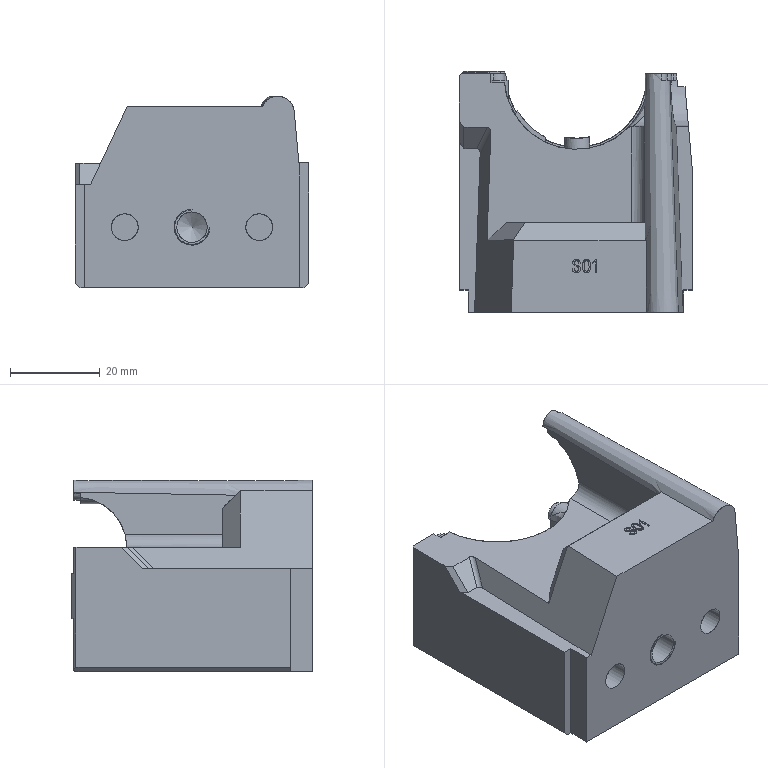NC program | PowerMill | posted with a generic post | part box 52 x 53.756 x 42.711 mm
Lines 1 to 869 of 4346:
%
O0001
N104 ( POWERMILL CB  : 2026004.0)
N105 ( POST VER      : 2026.0.0.5161)
N106 ( OPTION FILE   : FANUC)
N107 ( OUTPUT WORKPLANE : 2)
N108 (  )
N109 ( TOOL LIST )
N110 (----------------------------------)
N111 ( NO. | ID   | DIA.| TIP RAD|LENGTH)
N112 (----------------------------------)
N113 (    1|D6_2_1| 6.0 |  0.0   |113.48)
N114 (----------------------------------)
N115 (  )
N116 ( NUMBER OF TOOLPATHS: 3.0 )
N117 ( ESTIMATED PROGRAM DURATION: 0 HOURS 2 MIN 26 SEC)
N118 (  )
N119 G00 G21 G80 G40 G17
N120 G90
N121 G54
N122 G53 Z0.0
N123 (---------------)
N124 ( START TOOLPATH : 07中光-D6-偏置平坦面 )
N125 (---------------)
N126 ( TOOL NO.    :1 )
N127 ( TOOL TYPE   : ENDMILL)
N128 ( TOOL ID     : D6_2_1)
N129 ( TOOL DIA    : 6.0 LENGTH 113.48)
N130 T1
N131 M6
N132 S5000 M03
N133 G00 G90 X8.9124 Y5.3897
N134 G43 Z75.756 H1
N135
N136 G05 P10000 R8
N137 Z54.7966
N138 G01 Z51.7966 F720.0
N139 X11.893 Y6.4542 F1200.0
N140 G03 X12.572 Y7.201 I0.0994 J0.5917
N141 G01 X12.4998 Y7.4707
N142 X12.3858 Y8.1165
N143 X12.3489 Y8.7623
N144 X12.3871 Y9.4081
N145 X12.5024 Y10.0539
N146 X12.5902 Y10.3767
N147 X12.6965 Y10.6996
N148 X12.8294 Y11.0238
N149 X12.9822 Y11.3454
N150 X13.1662 Y11.6683
N151 G03 Y12.3141 I-0.5057 J0.3229
N152 G01 X13.1337 Y12.3688
N153 G03 X12.7655 Y12.6442 I-0.516 J-0.3061
N154 G00 Z61.4034
N155 G01 X18.2459 Y1.115 F10000.0
N156 G00 Z56.4034
N157 G01 Z53.4034 F720.0
N158 X18.309 Y1.1668 Z53.402
N159 X18.6189 Y1.5211 Z53.3937
N160 X18.8661 Y1.9216 Z53.3855
N161 X19.0441 Y2.3574 Z53.3773
N162 X19.148 Y2.8165 Z53.3691
N163 X19.1748 Y3.2864 Z53.3609
N164 X19.124 Y3.7544 Z53.3527
N165 X18.9968 Y4.2076 Z53.3445
N166 X18.7967 Y4.6337 Z53.3362
N167 X18.5293 Y5.021 Z53.328
N168 X18.2017 Y5.359 Z53.3198
N169 X17.823 Y5.6385 Z53.3116
N170 X17.4035 Y5.8519 Z53.3034
N171 X16.5943 Y6.1824 F1200.0
N172 G03 X15.2091 Y5.3093 I-0.3806 J-0.9316
N173 G01 X15.0298 Y2.2289
N174 G03 X17.3508 Y-0.1983 I2.2902 J-0.1334
N175 G01 X24.8762 Y-0.0974
N176 G03 X25.7346 Y0.2808 I-0.0161 J1.1999
N177 G01 X25.7821 Y0.3314
N178 G03 X26.1076 Y1.1529 I-0.8745 J0.8217
N179 G01 X26.1081 Y4.0803
N180 G03 X24.6739 Y5.2574 I-1.2 J0.0002
N181 G01 X24.3238 Y5.1877
N182 G02 X17.4035 Y5.8519 I-2.3558 J11.839
N183 G01 X18.4486 Y8.4106
N184 X18.2818 Y8.4796
N185 X17.9611 Y8.6531
N186 X17.7588 Y8.7865
N187 X17.5565 Y8.9418
N188 X17.3196 Y9.1568
N189 X17.0908 Y9.4081
N190 X16.8606 Y9.7215
N191 X16.6782 Y10.0349
N192 G03 X16.2538 Y10.3328 I-0.5231 J-0.2939
N193 G01 X16.0367 Y10.369
N194 X15.716 Y10.4468
N195 X15.3952 Y10.5508
N196 X15.0331 Y10.6996
N197 X14.7538 Y10.8428
N198 X14.433 Y11.0364
N199 X14.1123 Y11.2748
N200 X13.813 Y11.542
N201 G03 X13.0532 Y11.5825 I-0.4046 J-0.443
N202 G01 X13.0101 Y11.5509
N203 G00 Z61.3034
N204 G01 X32.0236 Y-1.2008 F10000.0
N205 G00 Z56.3034
N206 G01 Z53.3034 F720.0
N207 X28.9739 Y-0.3543 F1200.0
N208 X28.9897 Y-0.1775
N209 X28.9949 Y0.0
N210 Y10.584
N211 G03 X28.6905 Y10.2782 I0.2445 J-0.548
N212 G01 X28.5915 Y10.0539
N213 X28.4282 Y9.7648
N214 X28.1704 Y9.4081
N215 X27.8767 Y9.0936
N216 X27.5831 Y8.845
N217 X27.3972 Y8.7162
N218 X27.2053 Y8.5965
N219 X26.9416 Y8.4615
N220 X26.6209 Y8.3332
N221 X26.3002 Y8.2394
N222 X25.9794 Y8.1792
N223 X25.6587 Y8.1489
N224 X19.8855 Y8.1453
N225 X19.5648 Y8.1509
N226 X19.244 Y8.1846
N227 X18.9233 Y8.249
N228 X18.6026 Y8.3468
N229 X18.4486 Y8.4106
N230 X17.4035 Y5.8519
N231 G00 Z59.1251
N232 G01 X-26.9962 Y-5.6486 F10000.0
N233 G00 Z53.4274
N234 G01 Z50.4274 F720.0
N235 X-25.2713 Y-2.9949 F1200.0
N236 X-24.4645
N237 X-24.6756 Y-2.8617
N238 X-25.0172 Y-2.588
N239 X-25.206 Y-2.402
N240 X-25.3696 Y-2.216
N241 X-25.5257 Y-2.0108
N242 X-25.6587 Y-1.8057
N243 X-25.7884 Y-1.5702
N244 X-25.9311 Y-1.2473
N245 X-26.0361 Y-0.9244
N246 X-26.1083 Y-0.6015
N247 X-26.1493 Y-0.2786
N248 X-26.1613 Y0.0442
N249 X-26.1564 Y17.1574
N250 X-26.1259 Y17.4803
N251 X-26.0646 Y17.8032
N252 X-25.9709 Y18.1261
N253 X-25.8419 Y18.449
N254 X-25.6587 Y18.7958
N255 X-25.4569 Y19.0948
N256 X-25.2578 Y19.3362
N257 X-25.0172 Y19.5777
N258 X-24.8251 Y19.7406
N259 X-24.6047 Y19.9006
N260 X-24.3758 Y20.0417
N261 X-24.2982 Y20.0801
N262 G03 X-23.9656 Y20.575 I-0.2659 J0.5378
N263 G00 Z59.7966
N264 G01 X-29.2927 Y14.9242 F10000.0
N265 G00 Z54.7966
N266 G01 Z51.7966 F720.0
N267 X-26.1277 Y14.9179 F1200.0
N268 G03 X-25.7188 Y15.2435 I-0.132 J0.5853
N269 G01 X-25.5641 Y15.543
N270 X-25.3503 Y15.8659
N271 X-25.196 Y16.0589
N272 X-25.0172 Y16.2519
N273 X-24.7273 Y16.5117
N274 X-24.6136 Y16.5978
N275 G03 X-24.4207 Y16.8489 I-0.3625 J0.4782
N276 G01 X-24.2874 Y17.1574
N277 X-24.126 Y17.4803
N278 X-23.9341 Y17.8032
N279 X-23.7343 Y18.0965
N280 X-23.4543 Y18.449
N281 X-23.0928 Y18.8293
N282 X-22.7953 Y19.0948
N283 X-22.4514 Y19.3584
N284 X-22.1306 Y19.5712
N285 X-21.7927 Y19.7565
N286 X-21.4469 Y19.9268
N287 X-21.1684 Y20.037
N288 X-20.8477 Y20.1468
N289 X-20.527 Y20.2343
N290 X-19.8855 Y20.3516
N291 X-19.244 Y20.3926
N292 X-18.9628 Y20.3863
N293 X-18.6026 Y20.3592
N294 X-17.9611 Y20.252
N295 X-17.6404 Y20.1698
N296 X-17.3196 Y20.0651
N297 X-16.9989 Y19.9394
N298 X-16.5829 Y19.7406
N299 X-16.3574 Y19.6144
N300 X-16.0367 Y19.4101
N301 X-15.6189 Y19.0948
N302 X-15.3952 Y18.8942
N303 X-15.1333 Y18.6394
N304 X-14.9389 Y18.4201
N305 X-14.7538 Y18.193
N306 X-14.4806 Y17.8032
N307 G02 X-14.1117 Y17.1275 I-5.5646 J-3.4769
N308 G01 X-13.8711 Y16.5117
N309 X-13.7032 Y15.8659
N310 X-13.6155 Y15.2201
N311 X-13.6024 Y14.5743
N312 X-13.6644 Y13.9285
N313 X-13.7226 Y13.6056
N314 X-13.8041 Y13.2828
N315 X-13.9031 Y12.9599
N316 X-14.0501 Y12.5845
N317 G03 X-13.9801 Y11.9912 I0.5518 J-0.2357
N318 G01 X-13.7431 Y11.6683
N319 X-13.4708 Y11.2243
N320 X-13.2121 Y10.6996
N321 X-13.0839 Y10.3767
N322 X-12.9759 Y10.0539
N323 X-12.853 Y9.5472
N324 G03 X-12.6475 Y9.2224 I0.5831 J0.1415
N325 G00 Z61.3034
N326 G01 X-29.1579 Y7.8914 F10000.0
N327 G00 Z56.3034
N328 G01 Z53.3034 F720.0
N329 X-25.9929 F1200.0
N330 X-20.1653 Y7.8973
N331 X-20.1608 Y3.4188
N332 G03 X-19.5911 Y2.8625 I0.5571 J0.0006
N333 G01 X-18.9666 Y2.8767
N334 G03 X-18.3916 Y3.4867 I-0.0134 J0.5887
N335 G01 X-18.4764 Y5.8287
N336 G03 X-19.0964 Y8.9964 I-10.3124 J-0.3737
N337 G01 X-19.1874 Y9.2455
N338 G02 X-19.7746 Y11.8852 I9.6924 J3.5414
N339 G01 X-19.819 Y12.3914
N340 G03 X-20.1699 Y12.3759 I-0.1751 J-0.0153
N341 G01 X-20.1653 Y7.8973
N342 X-23.0827 Y7.8944
N343 X-23.0754 Y1.0916
N344 G03 X-21.8481 Y-0.1068 I1.2 J0.0013
N345 G01 X-16.7463 Y0.0094
N346 G03 X-15.7887 Y0.5235 I-0.0273 J1.1996
N347 G01 X-15.6927 Y0.6614
N348 G03 X-15.4776 Y1.3449 I-0.9849 J0.6855
N349 G01 X-15.469 Y6.4636
N350 G03 X-15.8506 Y8.7774 I-7.1317 J0.012
N351 G01 X-16.6899 Y11.2388
N352 G02 X-16.8362 Y12.8627 I3.2623 J1.1124
N353 G01 X-16.6534 Y14.0808
N354 G03 X-22.0119 Y15.5963 I-2.7758 J0.4166
N355 G01 X-22.8043 Y13.734
N356 G03 X-23.0875 Y12.3414 I3.2638 J-1.3888
N357 G01 X-23.0827 Y7.8944
N358 X-25.9929 Y7.8914
N359 G00 Z59.2944
N360 G01 X9.3033 Y28.856 F10000.0
N361 G00 Z54.2944
N362 G01 Z51.2944 F720.0
N363 X12.4055 Y28.2287 F1200.0
N364 G03 X12.6683 Y28.4498 I-0.2386 J0.5505
N365 G01 X12.9095 Y28.7815
N366 X13.1136 Y29.0299
N367 X13.3403 Y29.2784
N368 X13.4896 Y29.4272
N369 X13.801 Y29.7105
N370 X14.1123 Y29.9601
N371 X14.7051 Y30.3543
N372 X15.0745 Y30.5562
N373 X15.4014 Y30.7064
N374 X15.7341 Y30.8434
N375 X16.0913 Y30.9594
N376 G03 X16.4806 Y31.3176 I-0.17 J0.5755
N377 G00 Z59.7966
N378 G01 X10.034 Y19.3175 F10000.0
N379 G00 Z54.7966
N380 G01 Z51.7966 F720.0
N381 X12.6074 Y21.1599 F1200.0
N382 G03 X13.091 Y22.0439 I-0.044 J0.5984
N383 G01 X12.9396 Y22.3237
N384 X12.8294 Y22.5646
N385 X12.6665 Y22.9694
N386 X12.4829 Y23.6152
N387 X12.3777 Y24.261
N388 X12.3501 Y24.9068
N389 X12.3971 Y25.5526
N390 X12.4491 Y25.8755
N391 X12.5205 Y26.1983
N392 X12.6108 Y26.5212
N393 X12.7153 Y26.8119
N394 X12.8294 Y27.0989
N395 X13.0235 Y27.4899
N396 X13.2089 Y27.8128
N397 X13.4708 Y28.1937
N398 X13.682 Y28.4586
N399 X13.9807 Y28.7815
N400 X14.1123 Y28.9114
N401 X14.433 Y29.1902
N402 X14.7538 Y29.4323
N403 X15.0745 Y29.6356
N404 X15.3952 Y29.8182
N405 X16.0367 Y30.0982
N406 X16.4203 Y30.2223
N407 G03 X16.626 Y30.3452 I-0.1987 J0.5662
N408 G01 X16.9466 Y30.6023
N409 X17.1296 Y30.7226
N410 X17.3196 Y30.8317
N411 X17.4428 Y30.8894
N412 G03 X17.7762 Y31.312 I-0.2543 J0.5434
N413 G00 Z61.3034
N414 G01 X10.3441 Y20.3181 F10000.0
N415 G00 Z56.3034
N416 G01 Z53.3034 F720.0
N417 X13.0395 Y21.9768 F1200.0
N418 G03 X13.7919 Y22.0291 I0.3438 J0.4918
N419 G01 X14.1286 Y22.3237
N420 X14.4412 Y22.5536
N421 X14.7538 Y22.7418
N422 X15.0576 Y22.8962
N423 X15.3952 Y23.0338
N424 X15.716 Y23.1382
N425 X16.0367 Y23.216
N426 X16.1955 Y23.2423
N427 G03 X16.6458 Y23.5903 I-0.0979 J0.5919
N428 G01 X16.8389 Y23.9381
N429 X17.0711 Y24.261
N430 X17.3196 Y24.5361
N431 X17.6404 Y24.8192
N432 X17.7978 Y24.934
N433 X17.9611 Y25.0402
N434 X18.3225 Y25.2334
N435 X18.6026 Y25.3467
N436 X18.9233 Y25.444
N437 X19.244 Y25.5087
N438 X19.5648 Y25.5432
N439 X25.338 Y25.5484
N440 X25.6587 Y25.545
N441 X25.9794 Y25.5143
N442 X26.3002 Y25.4541
N443 X26.6209 Y25.3604
N444 X26.9416 Y25.2318
N445 X27.2225 Y25.087
N446 X27.5831 Y24.8481
N447 X27.8863 Y24.5903
N448 X28.0624 Y24.4099
N449 X28.2246 Y24.2169
N450 X28.4356 Y23.9161
N451 X28.6026 Y23.6152
N452 X28.6358 Y23.5384
N453 G03 X28.9949 Y23.2081 I0.5507 J0.2383
N454 G00 Z61.8056
N455 G01 X31.7425 Y16.7104 F10000.0
N456 G00 Z56.8056
N457 G01 Z53.8056 F720.0
N458 X28.5775 Y16.7105 F1200.0
N459 X22.8095 Y16.8427
N460 X22.8479 Y18.5202
N461 G03 X20.9327 Y19.5111 I-1.1996 J0.0276
N462 G01 X18.7565 Y17.8948
N463 G03 X18.2767 Y17.0369 I0.7155 J-0.9634
N464 G01 X18.2552 Y16.793
N465 G03 X18.7592 Y15.7067 I1.1953 J-0.1054
N466 G01 X20.88 Y14.2119
N467 G03 X22.771 Y15.1652 I0.6913 J0.9808
N468 G01 X22.8095 Y16.8427
N469 X25.6985 Y16.7765
N470 X25.7902 Y20.8875
N471 G03 X24.1888 Y22.5697 I-1.6456 J0.0367
N472 G01 X20.7571 Y22.6619
N473 G03 X19.8934 Y22.4415 I-0.0438 J-1.6304
N474 G01 X19.2223 Y22.0479
N475 X19.0912 Y21.945
N476 X18.7509 Y21.6373
N477 G02 X17.2364 Y20.5887 I-4.7835 J5.2909
N478 G01 X16.786 Y20.3565
N479 G03 X15.2339 Y17.9235 I1.3151 J-2.5505
N480 G01 X15.1498 Y15.8705
N481 G03 X16.4692 Y13.4819 I2.6267 J-0.1077
N482 G01 X17.7087 Y12.7716
N483 G02 X18.5121 Y12.2402 I-3.7476 J-6.5388
N484 G01 X19.2275 Y11.7055
N485 X20.0012 Y11.3242
N486 G03 X20.9079 Y11.11 I0.934 J1.9278
N487 G01 X24.0135 Y11.0704
N488 G03 X25.6055 Y12.6077 I0.02 J1.5723
N489 G01 X25.6985 Y16.7765
N490 X28.5775 Y16.7105
N491 G00 Z59.7966
N492 G01 X-8.6941 Y38.7527 F10000.0
N493 G00 Z54.7966
N494 G01 Z51.7966 F720.0
N495 X-11.8589 Y38.7903 F1200.0
N496 G03 X-12.2537 Y38.4682 I0.1461 J-0.582
N497 G01 X-12.4184 Y38.1453
N498 X-12.6593 Y37.783
N499 X-12.8294 Y37.5752
N500 X-13.0755 Y37.3242
N501 X-13.2459 Y37.1766
N502 X-13.4708 Y37.0088
N503 X-13.7916 Y36.8131
N504 X-13.8609 Y36.7782
N505 G03 X-14.0355 Y36.6456 I0.2694 J-0.536
N506 G01 X-14.1399 Y36.5308
N507 X-14.4468 Y36.2353
N508 X-14.7409 Y35.9873
N509 X-15.1362 Y35.7009
N510 X-15.3952 Y35.5439
N511 X-15.6987 Y35.3787
N512 X-16.0367 Y35.2248
N513 X-16.3574 Y35.1014
N514 X-16.6782 Y35.0002
N515 X-17.3196 Y34.8583
N516 X-17.9611 Y34.7934
N517 X-18.6026 Y34.8029
N518 X-19.244 Y34.8861
N519 X-19.5648 Y34.956
N520 X-19.8855 Y35.0482
N521 X-20.4048 Y35.2393
N522 X-20.8477 Y35.4507
N523 X-21.1684 Y35.6397
N524 X-21.5343 Y35.885
N525 X-21.8099 Y36.1026
N526 X-22.0379 Y36.306
N527 X-22.2659 Y36.5308
N528 G02 X-22.7953 Y37.1766 I4.2954 J4.0608
N529 G01 X-22.9485 Y37.4099
N530 X-23.0928 Y37.6489
N531 X-23.3404 Y38.1453
N532 X-23.4687 Y38.4682
N533 X-23.5777 Y38.791
N534 X-23.6635 Y39.1139
N535 X-23.7343 Y39.4772
N536 X-23.7763 Y39.7597
N537 X-23.8132 Y40.4055
N538 X-23.775 Y41.0513
N539 X-23.7343 Y41.3313
N540 X-23.6604 Y41.6971
N541 X-23.5731 Y42.0199
N542 G02 X-23.0928 Y43.1412 I5.3148 J-1.6129
N543 G01 X-22.9803 Y43.3386
N544 X-22.7973 Y43.6119
N545 X-22.6032 Y43.8775
N546 X-22.4322 Y44.0828
N547 X-22.2522 Y44.2802
N548 X-21.9737 Y44.5517
N549 X-21.7805 Y44.7285
N550 X-21.6126 Y44.926
N551 X-21.408 Y45.1356
N552 X-21.1768 Y45.335
N553 G03 X-20.9872 Y45.6409 I-0.3918 J0.4544
N554 G00 Z61.3034
N555 G01 X-9.0413 Y42.4574 F10000.0
N556 G00 Z56.3034
N557 G01 Z53.3034 F720.0
N558 X-12.0873 Y41.5977 F1200.0
N559 X-14.8561 Y41.053
N560 G03 X-15.9325 Y42.3068 I-1.6455 J-0.3238
N561 G01 X-16.3803 Y42.4675
N562 X-17.4041 Y42.7973
N563 G03 X-20.6393 Y40.2123 I-0.7614 J-2.3641
N564 G03 X-16.9972 Y38.2415 I2.4738 J0.2209
N565 G01 X-15.7451 Y38.9089
N566 G03 X-15.207 Y39.4941 I-0.5644 J1.059
N567 G01 X-14.9608 Y40.067
N568 G03 X-14.8561 Y41.053 I-1.5408 J0.6622
N569 G01 X-12.0873 Y41.5977
N570 G00 Z75.756
N571 G05 P0
N572 (---------------)
N573 ( END TOOLPATH : 07中光-D6-偏置平坦面 )
N574 (---------------)
N575 ( START TOOLPATH : 08中光-D6-等高 )
N576 (---------------)
N577 S3800 M03
N578 G00 X16.0016 Y22.9439 Z75.756
N579 G05 P10000 R8
N580 Z56.7743
N581 G01 Z53.7743 F1800.0
N582 G03 X16.6128 Y22.8331 I0.5124 J1.0851 F3000.0
N583 G01 X16.7904 Y22.8477
N584 G03 X16.8941 Y22.9286 I-0.0099 J0.1196
N585 G01 X17.044 Y23.2806
N586 X17.1284 Y23.4349
N587 X17.2489 Y23.6267
N588 X17.4745 Y23.9213
N589 X17.8207 Y24.2568
N590 X17.8955 Y24.3189
N591 X18.1668 Y24.5076
N592 X18.5129 Y24.6915
N593 X18.859 Y24.8231
N594 X19.2051 Y24.9076
N595 X19.5513 Y24.9539
N596 X19.8974 Y24.9611
N597 X25.0891 Y24.9597
N598 X25.4353 Y24.9292
N599 X25.6815 Y24.8845
N600 X25.8022 Y24.8501
N601 G03 X26.4233 Y24.8407 I0.3282 J1.1543
N602 G01 X26.4307 Y24.8425
N603 X26.4678 Y24.8615 Z53.7622
N604 X26.4819 Y24.8892 Z53.7319
N605 X26.4817 Y24.8957 Z53.7236
N606 X26.463 Y24.9161 Z53.69
N607 X26.422 Y24.9139 Z53.6753
N608 G02 X25.8022 Y24.8724 I-0.3873 J1.1357
N609 G01 X25.4353 Y24.9448
N610 X25.0891 Y24.9653
N611 X19.8974
N612 X19.5513 Y24.9576
N613 X19.2051 Y24.9131
N614 X18.859 Y24.827
N615 X18.4472 Y24.665
N616 X18.1668 Y24.5119
N617 X17.8207 Y24.2637
N618 X17.4745 Y23.9272
N619 X17.2423 Y23.6267
N620 X17.1284 Y23.4453
N621 X17.0395 Y23.2806
N622 X16.8918 Y22.9334
N623 G02 X16.7828 Y22.8521 I-0.1136 J0.0386
N624 G01 X16.6067 Y22.8378
N625 G02 X15.9956 Y22.9494 I-0.0972 J1.196
N626 G01 X15.964 Y22.9642 Z53.6607
N627 X15.9509 Y22.97 Z53.6257
N628 Z53.6254
N629 X15.964 Y22.9634 Z53.5906
N630 X15.9955 Y22.9484 Z53.5762
N631 X15.9958 Y22.9483
N632 G03 X16.607 Y22.8375 I0.5122 J1.0851
N633 G01 X16.7825 Y22.8521
N634 G03 X16.8918 Y22.9334 I-0.0043 J0.1199
N635 G01 X17.0395 Y23.2806
N636 X17.1284 Y23.4454
N637 X17.2423 Y23.6267
N638 X17.5154 Y23.9728
N639 X17.8207 Y24.2637
N640 X18.1668 Y24.5119
N641 X18.5129 Y24.6956
N642 X18.859 Y24.827
N643 X19.2051 Y24.9131
N644 X19.5513 Y24.9577
N645 X19.8974 Y24.9653
N646 X25.0891
N647 X25.4353 Y24.9546
N648 X25.8022 Y24.8945
N649 G03 X26.4203 Y24.9562 I0.194 J1.1842
N650 G01 X26.4254 Y24.9581
N651 X26.4569 Y24.9753 Z53.5635
N652 X26.4688 Y24.9928 Z53.5319
N653 X26.4686 Y24.995 Z53.5264
N654 X26.4529 Y25.0028 Z53.4919
N655 X26.4181 Y24.9945 Z53.4771
N656 G02 X25.8022 Y24.9136 I-0.459 J1.1087
N657 G01 X25.4353 Y24.9619
N658 X19.8974 Y24.9653
N659 X19.5513 Y24.9577
N660 X19.2051 Y24.9132
N661 X18.859 Y24.8271
N662 X18.4472 Y24.665
N663 X18.1668 Y24.5119
N664 X17.8207 Y24.2637
N665 X17.4745 Y23.9272
N666 X17.2423 Y23.6267
N667 X17.1284 Y23.4454
N668 X17.0395 Y23.2806
N669 X16.8918 Y22.9335
N670 G02 X16.7827 Y22.8521 I-0.1136 J0.0385
N671 G01 X16.6072 Y22.8374
N672 G02 X15.9959 Y22.9474 I-0.1003 J1.1958
N673 G01 X15.9642 Y22.9622 Z53.4626
N674 X15.9511 Y22.9682 Z53.4275
N675 Z53.4274
N676 X15.9642 Y22.9619 Z53.3925
N677 X15.9958 Y22.9469 Z53.378
N678 X15.9959
N679 G03 X16.6073 Y22.8373 I0.5102 J1.0861
N680 G01 X16.7815 Y22.852
N681 G03 X16.8853 Y22.9338 I-0.0101 J0.1196
N682 G01 X17.0291 Y23.2806
N683 X17.1284 Y23.4655
N684 X17.2277 Y23.6267
N685 X17.4951 Y23.9728
N686 X17.8602 Y24.3189
N687 X18.1668 Y24.5352
N688 X18.399 Y24.665
N689 X18.5129 Y24.72
N690 X18.859 Y24.8513
N691 X19.2051 Y24.9376
N692 X19.5513 Y24.9828
N693 X19.8974 Y24.9899
N694 X25.4353
N695 X25.8022 Y24.9566
N696 G03 X26.4143 Y25.0624 I0.1086 J1.195
N697 G00 Z58.8505
N698 G01 X26.4229 Y8.9145 F10000.0
N699 G00 Z56.7743
N700 G01 Z53.7743 F1800.0
N701 G03 X25.8022 Y8.9387 I-0.3554 J-1.1462 F3000.0
N702 G01 X25.4353 Y8.8555
N703 X25.0891 Y8.8258
N704 X19.8974 Y8.8246
N705 X19.5513 Y8.8316
N706 X19.2051 Y8.8772
N707 X18.859 Y8.9632
N708 X18.5232 Y9.0897
N709 X18.1668 Y9.2782
N710 X17.9359 Y9.4358
N711 X17.8207 Y9.5259
N712 X17.5487 Y9.782
N713 X17.4745 Y9.8632
N714 X17.2677 Y10.1281
N715 X17.1284 Y10.3471
N716 X16.9689 Y10.6655
N717 G03 X16.8653 Y10.7334 I-0.1082 J-0.052
N718 G01 X16.6123 Y10.7508
N719 G03 X16.0027 Y10.6317 I-0.0825 J-1.1971
N720 G01 X16.0 Y10.6304
N721 X15.9696 Y10.6151 Z53.7609
N722 X15.956 Y10.6076 Z53.7278
N723 X15.9558 Y10.6074 Z53.7248
N724 X15.9675 Y10.6122 Z53.69
N725 X15.9982 Y10.6269 Z53.6753
N726 G02 X16.6076 Y10.7472 I0.5292 J-1.077
N727 G01 X16.8513 Y10.7309
N728 G02 X16.9572 Y10.6611 I-0.0031 J-0.12
N729 G01 X17.0433 Y10.4742
N730 X17.1284 Y10.3169
N731 X17.2474 Y10.1281
N732 X17.5221 Y9.782
N733 X17.8207 Y9.4981
N734 X17.8984 Y9.4358
N735 X18.1668 Y9.2498
N736 X18.5129 Y9.066
N737 X18.859 Y8.9344
N738 X19.2051 Y8.8483
N739 X19.5513 Y8.8037
N740 X19.8974 Y8.7961
N741 X25.0891
N742 X25.4353 Y8.8152
N743 X25.8022 Y8.8863
N744 G02 X26.4219 Y8.8426 I0.2284 J-1.1781
N745 G01 X26.4309 Y8.8395
N746 X26.465 Y8.8193 Z53.6635
N747 X26.4779 Y8.7934 Z53.6339
N748 X26.4777 Y8.7872 Z53.6253
N749 X26.4596 Y8.7695 Z53.5912
N750 X26.4201 Y8.7737 Z53.5762
N751 G03 X25.8022 Y8.8379 I-0.4287 J-1.1208
N752 G01 X25.4353 Y8.7793
N753 X25.0891 Y8.7696
N754 X19.8974
N755 X19.5513 Y8.7772
N756 X19.2051 Y8.8218
N757 X18.859 Y8.9079
N758 X18.5129 Y9.0394
N759 X18.407 Y9.0897
N760 X18.1668 Y9.2232
N761 X17.8207 Y9.4716
N762 X17.4745 Y9.8082
N763 X17.2295 Y10.1281
N764 X17.1284 Y10.2904
N765 X17.0303 Y10.4742
N766 X16.9463 Y10.6604
N767 G03 X16.8403 Y10.731 I-0.1094 J-0.0494
N768 G01 X16.608 Y10.7475
N769 G03 X15.9981 Y10.6298 I-0.0853 J-1.1969
N770 G01 X15.9666 Y10.615 Z53.5616
N771 X15.9535 Y10.6096 Z53.5266
N772 Z53.526
N773 X15.9664 Y10.6169 Z53.4914
N774 X15.9976 Y10.6323 Z53.4771
N775 X15.9981 Y10.6326
N776 G02 X16.6085 Y10.7479 I0.5203 J-1.0813
N777 G01 X16.8293 Y10.7313
N778 G02 X16.9363 Y10.6582 I-0.0035 J-0.12
N779 G01 X17.0174 Y10.4742
N780 X17.1284 Y10.2638
N781 X17.212 Y10.1281
N782 X17.4745 Y9.7817
N783 X17.8207 Y9.445
N784 X18.1668 Y9.1967
N785 X18.3552 Y9.0897
N786 X18.5129 Y9.0129
N787 X18.859 Y8.8813
N788 X19.2051 Y8.7952
N789 X19.5513 Y8.7506
N790 X19.7149 Y8.7436
N791 X25.4353 Y8.7464
N792 X25.9223 Y8.8081
N793 G02 X26.5377 Y8.724 I0.1507 J-1.1905
N794 G01 X26.5782 Y8.6808 Z53.4615
N795 X26.5643 Y8.6311 Z53.4286
N796 X26.5435 Y8.6126 Z53.4124
N797 X26.4944 Y8.5924 Z53.3875
N798 X26.4376 Y8.6032 Z53.378
N799 X26.4123 Y8.6155
N800 G03 X25.8022 Y8.7325 I-0.5234 J-1.0799
N801 G01 X25.4353 Y8.7059
N802 X19.8974 Y8.7057
N803 X19.5513 Y8.7135
N804 X19.2051 Y8.7582
N805 X18.859 Y8.8444
N806 X18.5129 Y8.9761
N807 X18.287 Y9.0897
N808 X18.1668 Y9.16
N809 X17.7888 Y9.4358
N810 X17.4435 Y9.782
N811 X17.1894 Y10.1281
N812 X17.1284 Y10.2288
N813 X17.0008 Y10.4742
N814 X16.9246 Y10.6536
N815 G03 X16.8161 Y10.7315 I-0.1124 J-0.042
N816 G01 X16.6088 Y10.7481
N817 G03 X15.9979 Y10.6359 I-0.0961 J-1.1961
N818 G00 Z75.756
N819 G05 P0
N820 (---------------)
N821 ( END TOOLPATH : 08中光-D6-等高 )
N822 (---------------)
N823 ( START TOOLPATH : 25中光-D6-等高 )
N824 (---------------)
N825 G00 X-25.6231 Y-0.0466 Z75.756
N826 G05 P10000 R8
N827 Z56.258
N828 G01 Z53.258 F1800.0
N829 G03 X-25.4624 Y0.5534 I-1.0393 J0.6 F3000.0
N830 G01 X-25.4621 Y13.4321
N831 G03 X-25.6229 Y14.0321 I-1.2 J0.0001
N832 G01 X-25.6281 Y14.0413
N833 X-25.6439 Y14.069 Z53.2468
N834 X-25.6523 Y14.085 Z53.2183
N835 X-25.6533 Y14.0872 Z53.208
N836 X-25.6487 Y14.0809 Z53.1735
N837 X-25.6324 Y14.0534 Z53.1581
N838 G02 X-25.4716 Y13.4534 I-1.0392 J-0.6
N839 G01 Y0.5167
N840 G02 X-25.6324 Y-0.0833 I-1.2001 J0.0
N841 G01 X-25.6401 Y-0.0966
N842 X-25.6546 Y-0.1237 Z53.1483
N843 X-25.6621 Y-0.1418 Z53.1225
N844 X-25.6633 Y-0.1469 Z53.1081
N845 X-25.6579 Y-0.1443 Z53.0739
N846 X-25.6411 Y-0.1184 Z53.0581
N847 G03 X-25.4804 Y0.4816 I-1.0393 J0.6
N848 G01 Y13.474
N849 G03 X-25.6411 Y14.074 I-1.2 J0.0
N850 G01 X-25.6462 Y14.0827
N851 X-25.662 Y14.1106 Z53.0469
N852 X-25.6702 Y14.1266 Z53.018
N853 X-25.6711 Y14.1286 Z53.0082
N854 X-25.6663 Y14.1221 Z52.9736
N855 X-25.6499 Y14.0945 Z52.9582
N856 G02 X-25.4891 Y13.4945 I-1.0392 J-0.6
N857 G01 Y0.4464
N858 G02 X-25.6499 Y-0.1536 I-1.2 J0.0
N859 G01 X-25.6575 Y-0.1669
N860 X-25.6721 Y-0.194 Z52.9484
N861 X-25.6796 Y-0.2121 Z52.9226
N862 X-25.6808 Y-0.2172 Z52.9082
N863 X-25.6754 Y-0.2146 Z52.8741
N864 X-25.6586 Y-0.1887 Z52.8583
N865 G03 X-25.4979 Y0.4113 I-1.0393 J0.6
N866 G01 Y13.5151
N867 G03 X-25.6586 Y14.1151 I-1.2 J0.0
N868 G01 X-25.6637 Y14.1239
N869 X-25.6794 Y14.1518 Z52.847
N870 X-25.6877 Y14.1677 Z52.8182
N871 X-25.6886 Y14.1697 Z52.8083
N872 X-25.6838 Y14.1632 Z52.7737
N873 X-25.6674 Y14.1357 Z52.7584
N874 G02 X-25.5066 Y13.5357 I-1.0392 J-0.6
N875 G01 Y0.3761
N876 G02 X-25.6674 Y-0.2239 I-1.2 J0.0
N877 G01 X-25.675 Y-0.2372
N878 X-25.6896 Y-0.2643 Z52.7486
N879 X-25.6971 Y-0.2824 Z52.7228
N880 X-25.6983 Y-0.2875 Z52.7084
N881 X-25.6929 Y-0.2849 Z52.6743
N882 X-25.6761 Y-0.259 Z52.6584
N883 G03 X-25.5153 Y0.341 I-1.0393 J0.6
N884 G01 Y13.5563
N885 G03 X-25.6761 Y14.1563 I-1.2001 J0.0
N886 G01 X-25.6812 Y14.165
N887 X-25.6969 Y14.1929 Z52.6472
N888 X-25.7052 Y14.2088 Z52.6184
N889 X-25.7061 Y14.2109 Z52.6085
N890 X-25.7012 Y14.2044 Z52.5739
N891 X-25.6849 Y14.1768 Z52.5585
N892 G02 X-25.5241 Y13.5768 I-1.0392 J-0.6
N893 G01 Y0.3058
N894 G02 X-25.6849 Y-0.2942 I-1.2 J0.0
N895 G01 X-25.6925 Y-0.3075
N896 X-25.7071 Y-0.3346 Z52.5487
N897 X-25.7145 Y-0.3527 Z52.523
N898 X-25.7158 Y-0.3578 Z52.5086
N899 X-25.7104 Y-0.3552 Z52.4744
N900 X-25.6936 Y-0.3294 Z52.4586
N901 G03 X-25.5328 Y0.2706 I-1.0392 J0.6001
N902 G01 Y13.5974
N903 G03 X-25.6936 Y14.1974 I-1.2 J0.0
N904 G01 X-25.6987 Y14.2062
N905 X-25.7144 Y14.2341 Z52.4473
N906 X-25.7227 Y14.25 Z52.4185
N907 X-25.7236 Y14.252 Z52.4086
N908 X-25.7187 Y14.2455 Z52.374
N909 X-25.7023 Y14.218 Z52.3587
N910 G02 X-25.5416 Y13.618 I-1.0393 J-0.6
N911 G01 Y0.2355
N912 G02 X-25.7023 Y-0.3645 I-1.2 J0.0
N913 G01 X-25.71 Y-0.3778
N914 X-25.7246 Y-0.4049 Z52.3489
N915 X-25.732 Y-0.423 Z52.3231
N916 X-25.7333 Y-0.4281 Z52.3087
N917 X-25.7279 Y-0.4256 Z52.2746
N918 X-25.7111 Y-0.3997 Z52.2588
N919 G03 X-25.5503 Y0.2003 I-1.0392 J0.6
N920 G01 Y13.6385
N921 G03 X-25.7111 Y14.2385 I-1.2 J0.0
N922 G01 X-25.7161 Y14.2473
N923 X-25.7319 Y14.2752 Z52.2475
N924 X-25.7402 Y14.2911 Z52.2187
N925 X-25.741 Y14.2932 Z52.2088
N926 X-25.7362 Y14.2867 Z52.1742
N927 X-25.7198 Y14.2591 Z52.1588
N928 G02 X-25.559 Y13.6591 I-1.0393 J-0.6
N929 G01 Y0.1652
N930 G02 X-25.7198 Y-0.4348 I-1.2001 J0.0
N931 G01 X-25.7241 Y-0.4422
N932 X-25.7403 Y-0.4704 Z52.1471
N933 X-25.7489 Y-0.4856 Z52.1173
N934 X-25.7496 Y-0.4869 Z52.1089
N935 X-25.7449 Y-0.4792 Z52.0742
N936 X-25.7286 Y-0.4511 Z52.0589
N937 G03 X-25.5678 Y0.1489 I-1.0392 J0.6
N938 G01 Y13.6797
N939 G03 X-25.7286 Y14.2797 I-1.2 J0.0
N940 G01 X-25.7531 Y14.3222
N941 X-25.7661 Y14.3515 Z52.0536
N942 X-25.7713 Y14.3798 Z52.0383
N943 X-25.7727 Y14.4192 Z52.009
N944 X-25.7591 Y14.4357 Z51.9771
N945 X-25.7332 Y14.4137 Z51.959
N946 G02 X-25.5726 Y13.8137 I-1.0394 J-0.5997
N947 G01 X-25.5765 Y0.1461
N948 G02 X-25.7375 Y-0.4538 I-1.2 J0.0004
N949 G01 X-25.7391 Y-0.4567
N950 X-25.7569 Y-0.4859 Z51.9455
N951 X-25.7666 Y-0.4986 Z51.9123
N952 X-25.7668 Y-0.4987 Z51.909
N953 X-25.7624 Y-0.4868 Z51.8739
N954 X-25.746 Y-0.4567 Z51.8591
N955 G03 X-25.5853 Y0.1433 I-1.0393 J0.6
N956 G01 Y13.6852
N957 X-25.5748 Y14.0313
N958 X-25.526 Y14.3774
N959 X-25.4385 Y14.7113
N960 G03 X-25.4419 Y15.3325 I-1.1608 J0.3042
N961 G01 X-25.6351 Y16.0378
N962 X-25.6451 Y16.0721 Z51.8585
N963 X-25.6563 Y16.1061 Z51.8567
N964 X-25.8868 Y16.7723 Z51.8099
N965 X-25.8884 Y16.819 Z51.8023
N966 X-25.8491 Y16.8652 Z51.7822